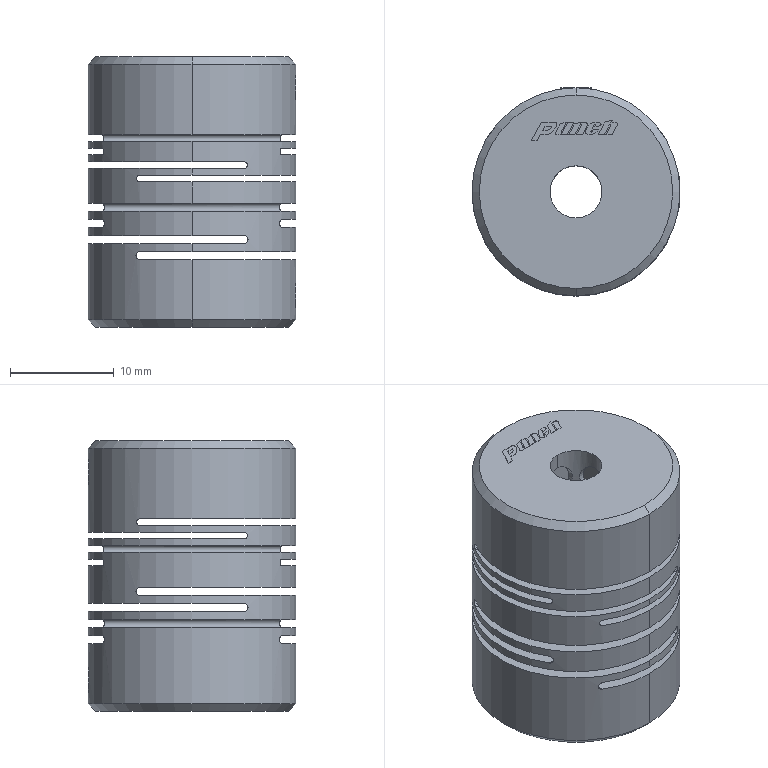Part | SolidWorks | features BaseBody 5 | 5 solids | 173 faces | box 20 x 20 x 26 mm | volume 5734 mm3 | plane 99 | cylinder 70 | cone 4 | commonest cylinder face diameters 3 x16 9.6 x14 20 x6 0.132 x5 0.647 x4 0.772 x4